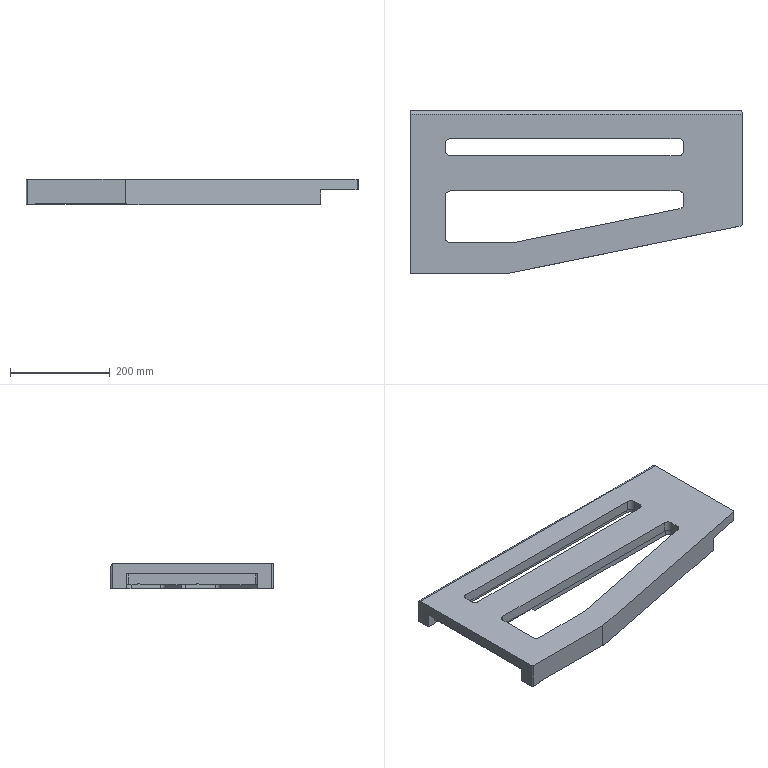Part | 1 solid | 73 faces | box 667 x 326 x 51 mm | volume 4744398 mm3 | plane 43 | cylinder 30 | commonest cylinder face diameters 19 x18 5 x5 17 x4 10 x2 14 x1